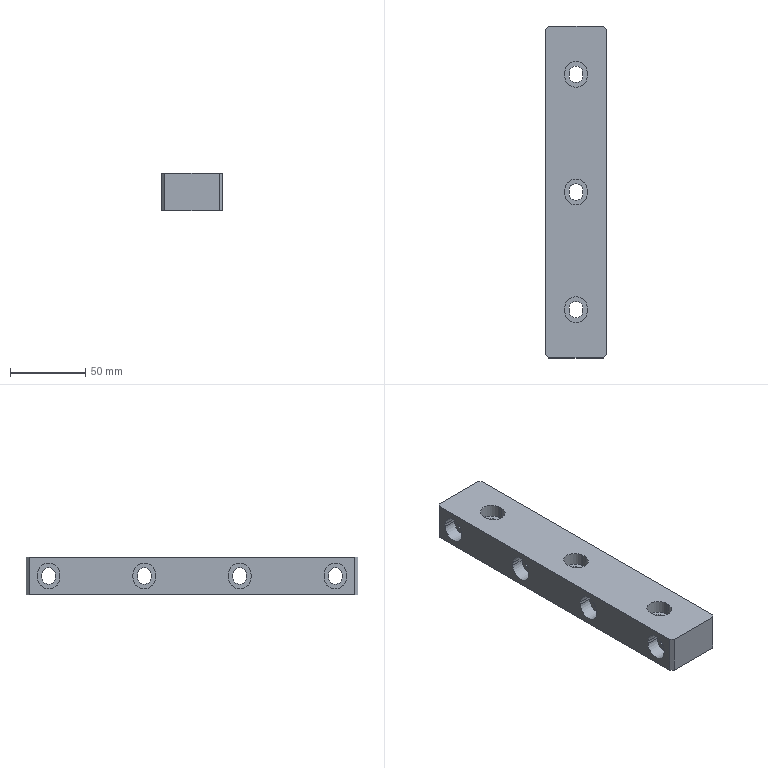Part | SolidWorks | features HoleWzd 2, Chamfer 1, Extrusion 1 | 1 solid | 81 faces | box 40 x 220 x 25 mm | volume 193089 mm3 | plane 45 | cylinder 36 | commonest cylinder face diameters 9 x18 15 x18